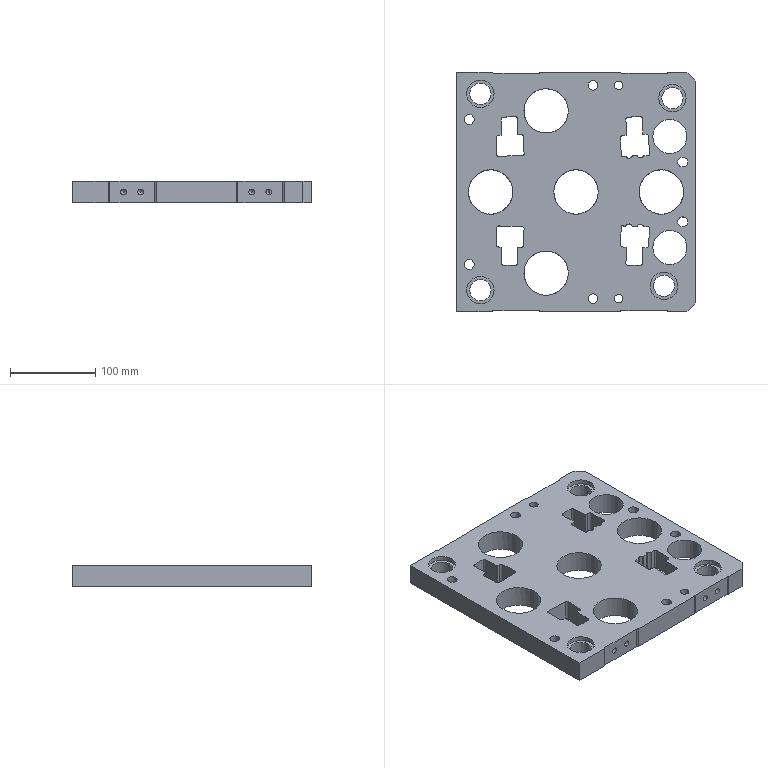Part | NX | features PH-12 2 | 1 solid | 163 faces | box 280 x 280 x 25 mm | volume 1407890 mm3 | cylinder 85 | plane 62 | cone 8 | spline 8 | commonest cylinder face diameters 4 x20 1 x16 6 x8 6.806 x8 11.5 x6 18 x6